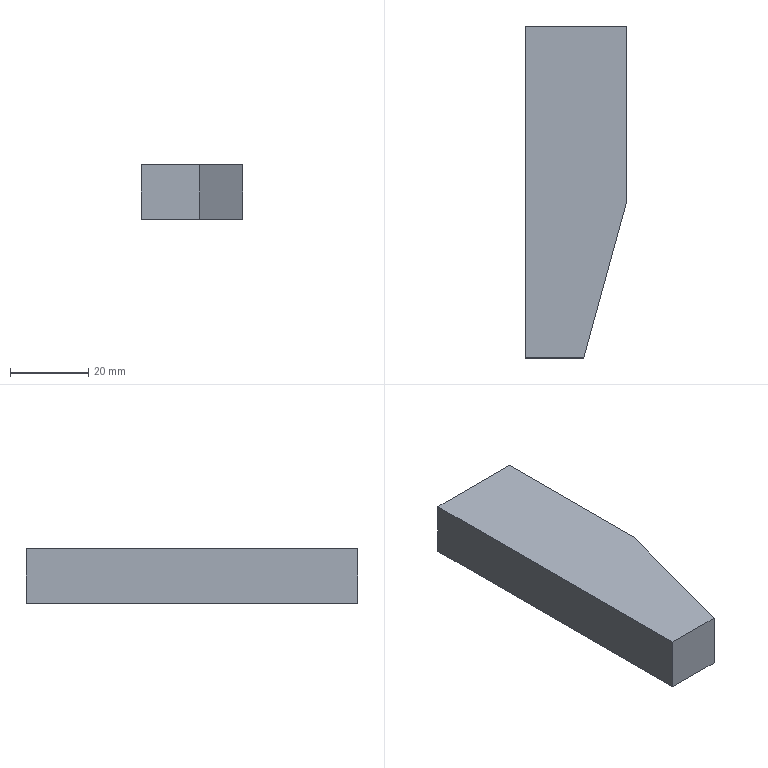Part | SolidWorks | features Extrusion 1 | 1 solid | 7 faces | box 26 x 85 x 14 mm | volume 27860 mm3 | plane 7
STEP:
#1=CARTESIAN_POINT('',(0.,0.,-7.));
#2=VERTEX_POINT('',#1);
#3=CARTESIAN_POINT('',(15.,0.,-7.));
#4=VERTEX_POINT('',#3);
#5=CARTESIAN_POINT('',(15.,0.,-7.));
#6=DIRECTION('',(1.,0.,0.));
#7=VECTOR('',#6,1000.);
#8=LINE('',#5,#7);
#9=EDGE_CURVE('',#2,#4,#8,.T.);
#10=ORIENTED_EDGE('',*,*,#9,.T.);
#11=CARTESIAN_POINT('',(15.,0.,7.));
#12=VERTEX_POINT('',#11);
#13=CARTESIAN_POINT('',(15.,0.,7.));
#14=DIRECTION('',(0.,0.,-1.));
#15=VECTOR('',#14,1000.);
#16=LINE('',#13,#15);
#17=EDGE_CURVE('',#12,#4,#16,.T.);
#18=ORIENTED_EDGE('',*,*,#17,.F.);
#19=CARTESIAN_POINT('',(0.,0.,7.));
#20=VERTEX_POINT('',#19);
#21=CARTESIAN_POINT('',(15.,0.,7.));
#22=DIRECTION('',(1.,0.,0.));
#23=VECTOR('',#22,1000.);
#24=LINE('',#21,#23);
#25=EDGE_CURVE('',#20,#12,#24,.T.);
#26=ORIENTED_EDGE('',*,*,#25,.F.);
#27=CARTESIAN_POINT('',(0.,0.,7.));
#28=DIRECTION('',(0.,0.,-1.));
#29=VECTOR('',#28,1000.);
#30=LINE('',#27,#29);
#31=EDGE_CURVE('',#20,#2,#30,.T.);
#32=ORIENTED_EDGE('',*,*,#31,.T.);
#33=EDGE_LOOP('',(#10,#18,#26,#32));
#34=FACE_OUTER_BOUND('',#33,.T.);
#35=CARTESIAN_POINT('',(15.,0.,7.));
#36=DIRECTION('',(0.,1.,0.));
#37=DIRECTION('',(0.,0.,1.));
#38=AXIS2_PLACEMENT_3D('',#35,#36,#37);
#39=PLANE('',#38);
#40=ADVANCED_FACE('',(#34),#39,.F.);
#41=CARTESIAN_POINT('',(26.,40.,-7.));
#42=VERTEX_POINT('',#41);
#43=CARTESIAN_POINT('',(26.,40.,-7.));
#44=DIRECTION('',(0.2652,0.9642,0.));
#45=VECTOR('',#44,1000.);
#46=LINE('',#43,#45);
#47=EDGE_CURVE('',#4,#42,#46,.T.);
#48=ORIENTED_EDGE('',*,*,#47,.T.);
#49=CARTESIAN_POINT('',(26.,40.,7.));
#50=VERTEX_POINT('',#49);
#51=CARTESIAN_POINT('',(26.,40.,7.));
#52=DIRECTION('',(0.,0.,-1.));
#53=VECTOR('',#52,1000.);
#54=LINE('',#51,#53);
#55=EDGE_CURVE('',#50,#42,#54,.T.);
#56=ORIENTED_EDGE('',*,*,#55,.F.);
#57=CARTESIAN_POINT('',(26.,40.,7.));
#58=DIRECTION('',(0.2652,0.9642,0.));
#59=VECTOR('',#58,1000.);
#60=LINE('',#57,#59);
#61=EDGE_CURVE('',#12,#50,#60,.T.);
#62=ORIENTED_EDGE('',*,*,#61,.F.);
#63=ORIENTED_EDGE('',*,*,#17,.T.);
#64=EDGE_LOOP('',(#48,#56,#62,#63));
#65=FACE_OUTER_BOUND('',#64,.T.);
#66=CARTESIAN_POINT('',(26.,40.,7.));
#67=DIRECTION('',(-0.9642,0.2652,0.));
#68=DIRECTION('',(-0.2652,-0.9642,0.));
#69=AXIS2_PLACEMENT_3D('',#66,#67,#68);
#70=PLANE('',#69);
#71=ADVANCED_FACE('',(#65),#70,.F.);
#72=CARTESIAN_POINT('',(26.,85.,-7.));
#73=VERTEX_POINT('',#72);
#74=CARTESIAN_POINT('',(26.,40.,-7.));
#75=DIRECTION('',(0.,1.,0.));
#76=VECTOR('',#75,1000.);
#77=LINE('',#74,#76);
#78=EDGE_CURVE('',#42,#73,#77,.T.);
#79=ORIENTED_EDGE('',*,*,#78,.T.);
#80=CARTESIAN_POINT('',(26.,85.,7.));
#81=VERTEX_POINT('',#80);
#82=CARTESIAN_POINT('',(26.,85.,7.));
#83=DIRECTION('',(0.,0.,-1.));
#84=VECTOR('',#83,1000.);
#85=LINE('',#82,#84);
#86=EDGE_CURVE('',#81,#73,#85,.T.);
#87=ORIENTED_EDGE('',*,*,#86,.F.);
#88=CARTESIAN_POINT('',(26.,40.,7.));
#89=DIRECTION('',(0.,1.,0.));
#90=VECTOR('',#89,1000.);
#91=LINE('',#88,#90);
#92=EDGE_CURVE('',#50,#81,#91,.T.);
#93=ORIENTED_EDGE('',*,*,#92,.F.);
#94=ORIENTED_EDGE('',*,*,#55,.T.);
#95=EDGE_LOOP('',(#79,#87,#93,#94));
#96=FACE_OUTER_BOUND('',#95,.T.);
#97=CARTESIAN_POINT('',(26.,40.,7.));
#98=DIRECTION('',(-1.,0.,0.));
#99=DIRECTION('',(0.,-1.,0.));
#100=AXIS2_PLACEMENT_3D('',#97,#98,#99);
#101=PLANE('',#100);
#102=ADVANCED_FACE('',(#96),#101,.F.);
#103=CARTESIAN_POINT('',(0.,85.,-7.));
#104=VERTEX_POINT('',#103);
#105=CARTESIAN_POINT('',(0.,85.,-7.));
#106=DIRECTION('',(-1.,0.,0.));
#107=VECTOR('',#106,1000.);
#108=LINE('',#105,#107);
#109=EDGE_CURVE('',#73,#104,#108,.T.);
#110=ORIENTED_EDGE('',*,*,#109,.T.);
#111=CARTESIAN_POINT('',(0.,85.,7.));
#112=VERTEX_POINT('',#111);
#113=CARTESIAN_POINT('',(0.,85.,7.));
#114=DIRECTION('',(0.,0.,-1.));
#115=VECTOR('',#114,1000.);
#116=LINE('',#113,#115);
#117=EDGE_CURVE('',#112,#104,#116,.T.);
#118=ORIENTED_EDGE('',*,*,#117,.F.);
#119=CARTESIAN_POINT('',(0.,85.,7.));
#120=DIRECTION('',(-1.,0.,0.));
#121=VECTOR('',#120,1000.);
#122=LINE('',#119,#121);
#123=EDGE_CURVE('',#81,#112,#122,.T.);
#124=ORIENTED_EDGE('',*,*,#123,.F.);
#125=ORIENTED_EDGE('',*,*,#86,.T.);
#126=EDGE_LOOP('',(#110,#118,#124,#125));
#127=FACE_OUTER_BOUND('',#126,.T.);
#128=CARTESIAN_POINT('',(0.,85.,7.));
#129=DIRECTION('',(0.,-1.,0.));
#130=DIRECTION('',(0.,0.,-1.));
#131=AXIS2_PLACEMENT_3D('',#128,#129,#130);
#132=PLANE('',#131);
#133=ADVANCED_FACE('',(#127),#132,.F.);
#134=CARTESIAN_POINT('',(0.,0.,-7.));
#135=DIRECTION('',(0.,-1.,0.));
#136=VECTOR('',#135,1000.);
#137=LINE('',#134,#136);
#138=EDGE_CURVE('',#104,#2,#137,.T.);
#139=ORIENTED_EDGE('',*,*,#138,.T.);
#140=ORIENTED_EDGE('',*,*,#31,.F.);
#141=CARTESIAN_POINT('',(0.,0.,7.));
#142=DIRECTION('',(0.,-1.,0.));
#143=VECTOR('',#142,1000.);
#144=LINE('',#141,#143);
#145=EDGE_CURVE('',#112,#20,#144,.T.);
#146=ORIENTED_EDGE('',*,*,#145,.F.);
#147=ORIENTED_EDGE('',*,*,#117,.T.);
#148=EDGE_LOOP('',(#139,#140,#146,#147));
#149=FACE_OUTER_BOUND('',#148,.T.);
#150=CARTESIAN_POINT('',(0.,0.,7.));
#151=DIRECTION('',(1.,0.,0.));
#152=DIRECTION('',(0.,1.,0.));
#153=AXIS2_PLACEMENT_3D('',#150,#151,#152);
#154=PLANE('',#153);
#155=ADVANCED_FACE('',(#149),#154,.F.);
#156=ORIENTED_EDGE('',*,*,#25,.T.);
#157=ORIENTED_EDGE('',*,*,#61,.T.);
#158=ORIENTED_EDGE('',*,*,#92,.T.);
#159=ORIENTED_EDGE('',*,*,#123,.T.);
#160=ORIENTED_EDGE('',*,*,#145,.T.);
#161=EDGE_LOOP('',(#156,#157,#158,#159,#160));
#162=FACE_OUTER_BOUND('',#161,.T.);
#163=CARTESIAN_POINT('',(0.,0.,7.));
#164=DIRECTION('',(0.,0.,-1.));
#165=DIRECTION('',(-1.,0.,0.));
#166=AXIS2_PLACEMENT_3D('',#163,#164,#165);
#167=PLANE('',#166);
#168=ADVANCED_FACE('',(#162),#167,.F.);
#169=ORIENTED_EDGE('',*,*,#9,.F.);
#170=ORIENTED_EDGE('',*,*,#138,.F.);
#171=ORIENTED_EDGE('',*,*,#109,.F.);
#172=ORIENTED_EDGE('',*,*,#78,.F.);
#173=ORIENTED_EDGE('',*,*,#47,.F.);
#174=EDGE_LOOP('',(#169,#170,#171,#172,#173));
#175=FACE_OUTER_BOUND('',#174,.T.);
#176=CARTESIAN_POINT('',(0.,0.,-7.));
#177=DIRECTION('',(0.,0.,-1.));
#178=DIRECTION('',(-1.,0.,0.));
#179=AXIS2_PLACEMENT_3D('',#176,#177,#178);
#180=PLANE('',#179);
#181=ADVANCED_FACE('',(#175),#180,.T.);
#182=CLOSED_SHELL('',(#40,#71,#102,#133,#155,#168,#181));
#183=MANIFOLD_SOLID_BREP('',#182);
#184=CARTESIAN_POINT('',(0.,0.,0.));
#185=DIRECTION('',(0.,0.,1.));
#186=DIRECTION('',(1.,0.,0.));
#187=AXIS2_PLACEMENT_3D('',#184,#185,#186);
#188=(LENGTH_UNIT()NAMED_UNIT(*)SI_UNIT(.MILLI.,.METRE.));
#189=UNCERTAINTY_MEASURE_WITH_UNIT(LENGTH_MEASURE(0.00001),#188,'','');
#190=(NAMED_UNIT(*)PLANE_ANGLE_UNIT()SI_UNIT($,.RADIAN.));
#191=(NAMED_UNIT(*)SI_UNIT($,.STERADIAN.)SOLID_ANGLE_UNIT());
#192=(GEOMETRIC_REPRESENTATION_CONTEXT(3)GLOBAL_UNCERTAINTY_ASSIGNED_CONTEXT((#189))GLOBAL_UNIT_ASSIGNED_CONTEXT((#188,#190,#191))REPRESENTATION_CONTEXT('',''));
#193=ADVANCED_BREP_SHAPE_REPRESENTATION('',(#183,#187),#192);